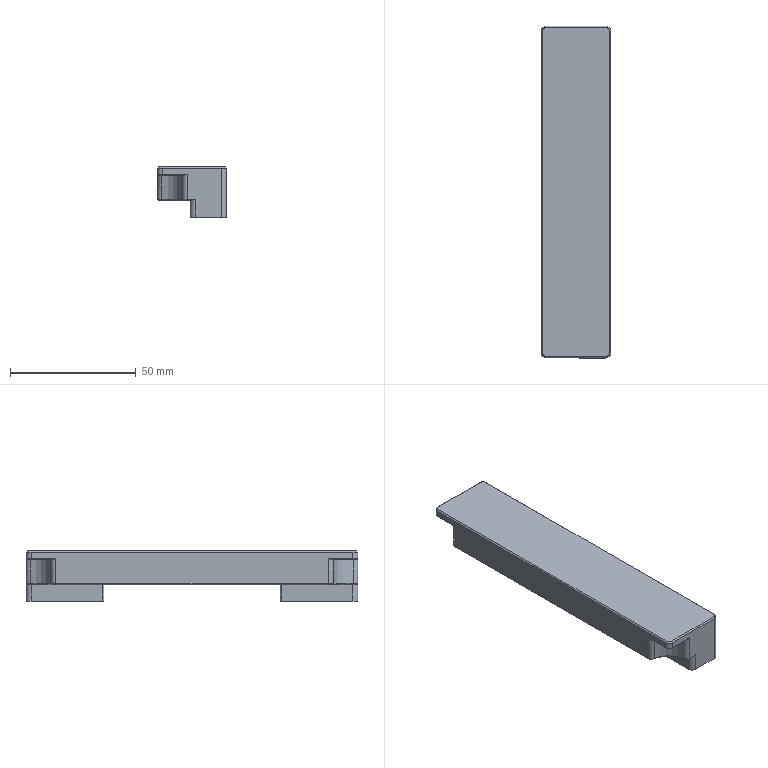Part | 1 solid | 77 faces | box 27.5 x 132 x 20 mm | volume 41660 mm3 | plane 33 | cylinder 24 | cone 20 | commonest cylinder face diameters 4 x14 6 x8 20 x2